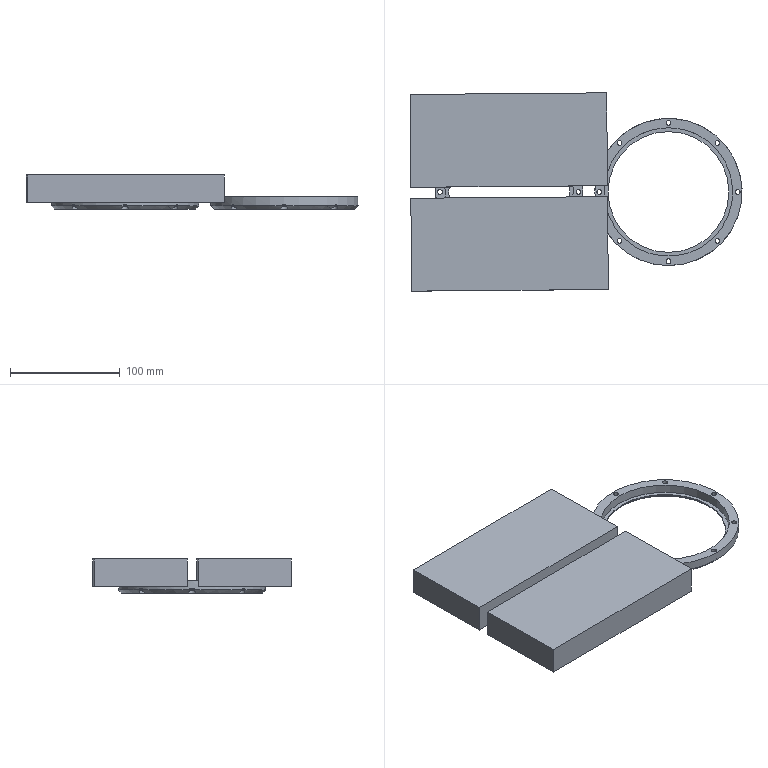CAM job | NX | 3-axis milling, drilling | part box 302.234 x 180.468 x 31 mm
Tools:
number,name,description,diameter,corner_radius,flute_length,length,flutes
4,D4,平底铣刀-粗,4.0,0.0,25.0,75.0,2
9,D10,平底铣刀-粗,10.0,0.0,35.0,75.0,2
11,D4-J,平底铣刀-精,4.0,0.0,50.0,75.0,2
7,D6-J,平底铣刀-精,6.0,0.0,25.0,75.0,2
10,D10-J,平底铣刀-精,10.0,0.0,35.0,75.0,2
17,D6R0.5,圆鼻刀-粗,6.0,0.5,50.0,75.0,2
1,D80R0.8飞刀,圆鼻刀-粗,80.0,0.8,50.0,75.0,2
1,D80R0.8飞刀-J,圆鼻刀-精,80.0,0.8,50.0,75.0,2
2,D6倒角刀,倒角刀,6.0,0.0,3.0,25.0,2
14,ZT4.3,Drilling Tool,4.3,0.0,50.0,75.0,4
Operations:
program,operation,operation_type,tool,method,geometry_group,spindle_rpm,surface_speed,feed_per_tooth,feed_cut,feed_plunge,cut_length_mm,path_length_mm,cut_time_min,machine_time_min
C,FLOORWALL_LAYERROUGH-MED_COPY,VolumeBased25DMillingOperation,D10,LAYERROUGH-DOC_K-STEP_G,W-C,8000.0,251.32,0.25,4000.0,100.0,16976.481,17519.271,4.244,4.298
C,FLOORWALL_FINISHFLOOR-MED_COPY,VolumeBased25DMillingOperation,D10-J,FINISH-STEP-DOC_OFF,W-C,7000.0,175.0,0.0536,1500.0,100.0,2629.9,2657.2,1.753,1.756
C,C0.3_CLOSEDCONTOUR_CHAMFER6X45L_COPY,PlanarMilling,D6倒角刀,WALL_CHAMFER-DOC_0-STEP_G,W-C,7000.0,131.0,0.1071,1500.0,100.0,429.799,525.799,0.2865,0.2961
C,FLOORWALL_FINISHSIDE-MED-SELFLOOR_COPY,VolumeBased25DMillingOperation,D10-J,SIDEFINISH-DOC_K-STEP_G,W-C,8000.0,251.32,0.0625,1000.0,100.0,398.709,426.709,0.3987,0.4015
B,ZLEVEL_HELIXWALL_COPY,ZLevelMilling,D10,ZLEVELWALL-DOC_K-STEP_G,W-B,7000.0,219.911,0.2857,4000.0,100.0,5139.028,5238.028,1.285,1.295
B,ZLEVEL_HELIXWALL_COPY_COPY,ZLevelMilling,D10,ZLEVELWALL-DOC_K-STEP_G,W-B,7000.0,219.911,0.2857,4000.0,100.0,10259.965,10359.965,2.565,2.575
B,CENTERSPOT,Operation,D6倒角刀,METHOD,W-B,3000.0,56.549,0.0333,200.0,0.0,20.0,484.599,0.1,0.1465
B,DRILL,Operation,ZT4.3,METHOD,W-B,3000.0,40.526,0.01,120.0,0.0,114.336,673.27,0.9528,1.009
B,HOLEROUGH_1,CylinderMilling,D4,METHOD,W-B,6000.0,75.398,0.1,1200.0,100.0,1653.624,2820.752,1.378,1.495
B,HOLESIDE_1,CylinderMilling,D4-J,METHOD,W-B,6000.0,75.398,0.05,600.0,100.0,107.081,1308.61,0.1785,0.2986
B,MILLCHAMFER_1,PlanarMilling,D6倒角刀,METHOD,W-B,6000.0,113.097,0.05,600.0,100.0,644.547,1785.025,1.074,1.188
B,ZLEVEL_HELIXWALL_COPY_COPY_1,ZLevelMilling,D6R0.5,ZLEVELWALL-DOC_K-STEP_G,W-B,10000.0,188.496,0.225,4500.0,100.0,12350.01,12449.511,2.744,2.754
B,ZLEVEL_HELIXWALL_COPY_COPY_COPY,ZLevelMilling,D6R0.5,ZLEVELWALL-DOC_K-STEP_G,W-B,10000.0,188.496,0.225,4500.0,100.0,22064.464,22164.964,4.903,4.913
A,FLOORWALL_FACEROUGH_COPY,VolumeBased25DMillingOperation,D80R0.8飞刀,LAYERROUGH-DOC_K-STEP_G,W-A,4500.0,1130.973,0.2222,2000.0,100.0,2295.8,2769.098,1.148,1.195
A,FLOORWALL_FACEFINISH_COPY,VolumeBased25DMillingOperation,D80R0.8飞刀-J,SIDEFINISH-DOC_K-STEP_G,W-A,4000.0,1005.28,0.125,1000.0,100.0,1147.219,1243.219,1.147,1.157
A,FLOORWALL_HELIXROUGH-MED_COPY_COPY,VolumeBased25DMillingOperation,D10,LAYERROUGH-DOC_K-STEP_G,W-A,8000.0,251.32,0.25,4000.0,100.0,13209.336,13606.899,3.302,3.342
A,FLOORWALL_HELIXROUGH-MED_COPY,VolumeBased25DMillingOperation,D10,LAYERROUGH-DOC_K-STEP_G,W-A,8000.0,251.32,0.25,4000.0,100.0,10106.691,10444.473,2.527,2.561
A,OUTLINE_ROUGH_2,VolumeBased25DMillingOperation,D10,METHOD,W-A,6000.0,188.0,0.25,4000.0,80.0,21747.859,22110.359,5.437,5.473
A,CHAMFER_2,SurfaceContour,D6倒角刀,METHOD,W-A,6000.0,113.0,0.125,1200.0,100.0,2329.691,3689.36,1.941,2.077
A,FLOORWALL_FINISHSIDE-MED_COPY,VolumeBased25DMillingOperation,D6-J,SIDEFINISH-DOC_K-STEP_G,W-A,8000.0,150.792,0.0625,1000.0,100.0,1421.436,1698.024,1.421,1.449
A,ZSTOCK0.5_FLOORWALL_OFFSET0.1_RAMPFINISH-MED_COPY,VolumeBased25DMillingOperation,D6-J,SIDEFINISH-DOC_K-STEP_G,W-A,8000.0,150.792,0.0625,1000.0,100.0,694.863,1093.341,0.6949,0.7347
A,OUTLINE_SEMIFINISH_2,VolumeBased25DMillingOperation,D6-J,METHOD,W-A,6000.0,113.0,0.0833,1000.0,100.0,889.701,1358.732,0.8897,0.9366
A,OUTLINE_FINISH_2,VolumeBased25DMillingOperation,D6-J,METHOD,W-A,6000.0,113.0,0.0833,1000.0,100.0,889.301,1359.405,0.8893,0.9363